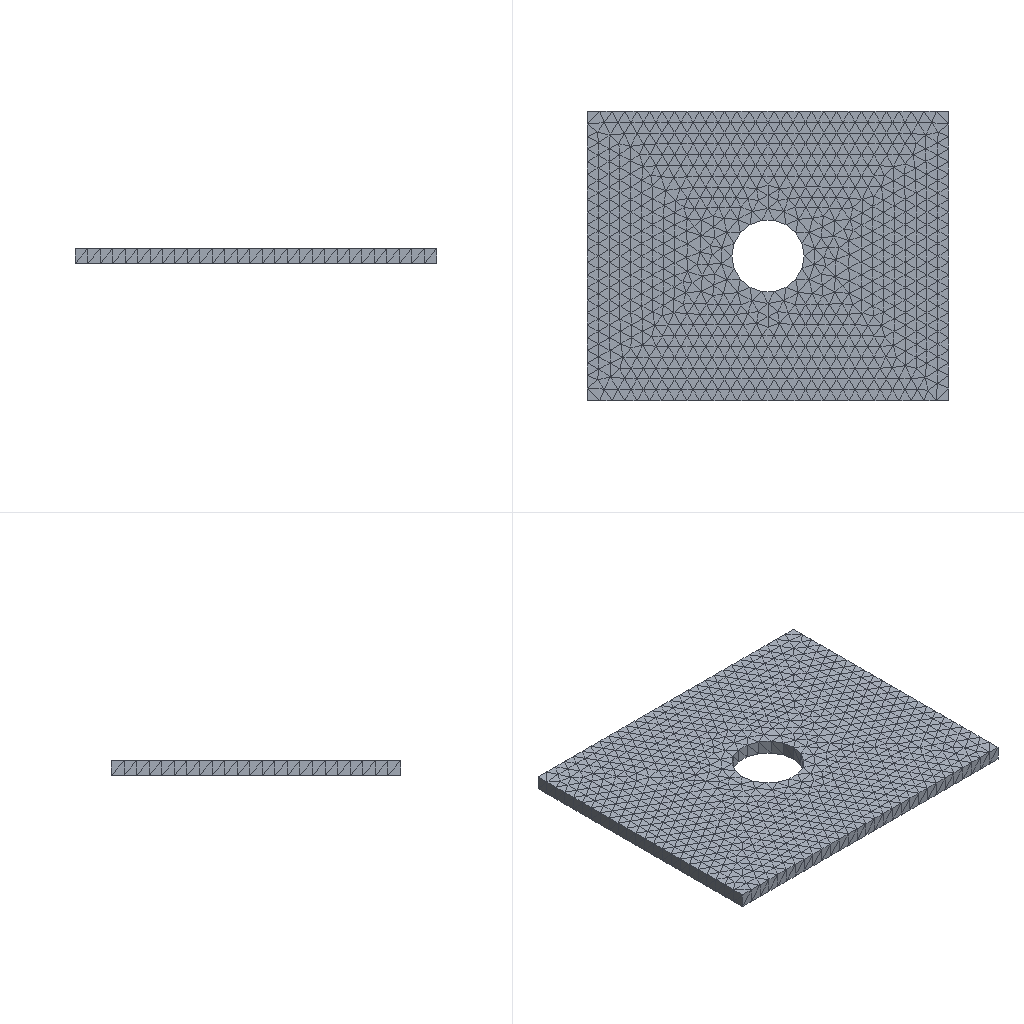Simulation study | abaqus
Notes in the study folder:
02 plate with hole
job_status=None
Umax_mm=0.00980797
S_Mises_max_MPa=15.475
Set-up summary:
category,name,step,type,value,unit,region
solver,abaqus,,Abaqus/CAE 2024
units,mm-N-s-tonne (MPa),,inferred,E=210000 density=7.85e-09
analysis,Step-1,,static,time_period=1
mesh,nodes,,,14651
mesh,elements,,,8511
element_type,C3D10,,,8511
material,Steel,,E,210000
material,Steel,,nu,0.3
material,Steel,,density,7.85e-09
section,Steel,,solid section,,,_PickedSet2
load,P,Step-1,pressure,0.1,,PRESS
bc,BC,Step-1,encastre,[dofs=ENCASTRE],,FIXED
Abaqus input file, long lists of numbers shortened:
*Heading
** Job name: deck Model name: M02
** Generated by: Abaqus/CAE 2024
*Preprint, echo=NO, model=NO, history=NO, contact=NO
**
** PARTS
**
*Part, name=P
*Node
      1,          50.,          40.,           4.
      2,          50.,         -40.,           4.
** (14649 more lines like these left out)
*Element, type=C3D10
   1,   578,  1593,  1594,  1595,  2277,  2276,  2275,  2279,  2278,  2280
   2,  1596,  1595,  1249,  1252,  2283,  2282,  2281,  2285,  2284,  2286
** (8509 more lines like these left out)
*Nset, nset=_PickedSet2, internal, generate
     1,  14651,      1
*Elset, elset=_PickedSet2, internal, generate
    1,  8511,     1
** Section: Sec
*Solid Section, elset=_PickedSet2, material=Steel
,
*End Part
**
**
** ASSEMBLY
**
*Assembly, name=Assembly
**
*Instance, name=I, part=P
*End Instance
**
*Nset, nset=FIXED, instance=I
     1,     2,     3,     4,     7,     8,     9,    10,    89,    90,    91,    92,    93,    94,    95,    96
    97,    98,    99,   100,   101,   102,   103,   104,   105,   106,   107,   108,   109,   110,   111,   112
** (21 more lines like these left out)
*Elset, elset=FIXED, instance=I
  807,  916,  926,  973, 1068, 1205, 1233, 1325, 1356, 2151, 2225, 2420, 2487, 2580, 2605, 2646
 2653, 2656, 2730, 2745, 3143, 3166, 3394, 3405, 3409, 3435, 3477, 3482, 3493, 3497, 3511, 3517
** (6 more lines like these left out)
*Elset, elset=_PRESS_S2, internal, instance=I
   98,  875,  911, 2823, 2946, 4386, 5693, 7234, 8075
*Elset, elset=_PRESS_S3, internal, instance=I
  228,  291,  381,  418,  466,  470,  476,  532,  551,  558,  563,  564,  572,  592,  600,  637
  648,  669,  670,  684,  713,  820,  826,  841,  863,  887,  888,  948,  952,  966,  974, 1002
** (88 more lines like these left out)
*Elset, elset=_PRESS_S4, internal, instance=I
  358, 1611, 2437, 2689, 3097, 3151, 3370, 3394, 3587, 4677, 4709, 4711, 4969, 5199, 5968, 6714
 7283, 7296, 8253, 8455
*Elset, elset=_PRESS_S1, internal, instance=I
 2194, 2346, 5089, 5289, 5685, 6004, 6644, 7913
*Surface, type=ELEMENT, name=PRESS
_PRESS_S2, S2
_PRESS_S3, S3
_PRESS_S4, S4
_PRESS_S1, S1
*End Assembly
**
** MATERIALS
**
*Material, name=Steel
*Density
 7.85e-09,
*Elastic
210000., 0.3
** ----------------------------------------------------------------
**
** STEP: Step-1
**
*Step, name=Step-1, nlgeom=NO
*Static
1., 1., 1e-05, 1.
**
** BOUNDARY CONDITIONS
**
** Name: BC Type: Symmetry/Antisymmetry/Encastre
*Boundary
FIXED, ENCASTRE
**
** LOADS
**
** Name: P   Type: Pressure
*Dsload
PRESS, P, 0.1
**
** OUTPUT REQUESTS
**
*Restart, write, frequency=0
**
** FIELD OUTPUT: F-Output-1
**
*Output, field, variable=PRESELECT
**
** HISTORY OUTPUT: H-Output-1
**
*Output, history, variable=PRESELECT
*End Step
Results summary:
result,odb.job_status,,,JOB_STATUS_COMPLETED_SUCCESSFULLY,"consistent, unstated (Abaqus has no unit system)"
result,steps[0].procedure,Step-1,,*STATIC,"consistent, unstated (Abaqus has no unit system)"
result,steps[0].time_period,Step-1,,1,"consistent, unstated (Abaqus has no unit system)"
result,steps[0].n_frames,Step-1,,2,"consistent, unstated (Abaqus has no unit system)"
result,steps[0].last_frame.id,Step-1,,1,"consistent, unstated (Abaqus has no unit system)"
result,steps[0].last_frame.value,Step-1,,1,"consistent, unstated (Abaqus has no unit system)"
result,steps[0].last_frame.description,Step-1,,Increment      1: Step Time =    1.000,"consistent, unstated (Abaqus has no unit system)"
result,steps[0].completed,Step-1,,True,"consistent, unstated (Abaqus has no unit system)"
result,steps[0].max_U_magnitude,Step-1,,0.009808,"consistent, unstated (Abaqus has no unit system)"
result,steps[0].max_S_mises,Step-1,,15.475,"consistent, unstated (Abaqus has no unit system)"
result,steps[0].RF_sum[1],Step-1,,-2.86102e-06,"consistent, unstated (Abaqus has no unit system)"
result,steps[0].RF_sum[2],Step-1,,0.0001774,"consistent, unstated (Abaqus has no unit system)"
result,steps[0].RF_sum[3],Step-1,,768.585,"consistent, unstated (Abaqus has no unit system)"
result,steps[1].procedure,Step-1,,*STATIC,"consistent, unstated (Abaqus has no unit system)"
result,steps[1].time_period,Step-1,,1,"consistent, unstated (Abaqus has no unit system)"
result,steps[1].n_frames,Step-1,,2,"consistent, unstated (Abaqus has no unit system)"
result,steps[1].last_frame.id,Step-1,,1,"consistent, unstated (Abaqus has no unit system)"
result,steps[1].last_frame.value,Step-1,,1,"consistent, unstated (Abaqus has no unit system)"
result,steps[1].last_frame.description,Step-1,,Increment      1: Step Time =    1.000,"consistent, unstated (Abaqus has no unit system)"
result,steps[1].completed,Step-1,,True,"consistent, unstated (Abaqus has no unit system)"
result,steps[1].max_U_magnitude,Step-1,,0.009808,"consistent, unstated (Abaqus has no unit system)"
result,steps[1].max_S_mises,Step-1,,15.475,"consistent, unstated (Abaqus has no unit system)"
result,steps[1].RF_sum[1],Step-1,,-2.86102e-06,"consistent, unstated (Abaqus has no unit system)"
result,steps[1].RF_sum[2],Step-1,,0.0001774,"consistent, unstated (Abaqus has no unit system)"
result,steps[1].RF_sum[3],Step-1,,768.585,"consistent, unstated (Abaqus has no unit system)"